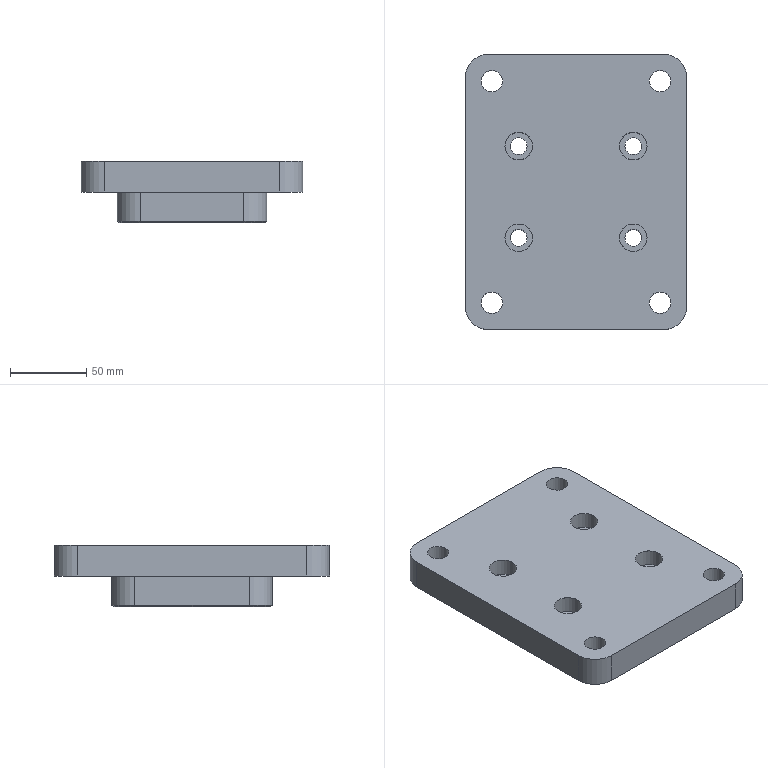NC program | NX | posted with a generic post | part box 145 x 180 x 40 mm
Whole program:
N10 G17 G21 G94 G90
(ZLEVEL_PROFILE_COPY_COPY , TOOL : D50)
N12 T02 M6
N14 G54
N16 G17 G0 G90 X-77.65 Y-31.479 S1200 M3
N18 G43 Z30. H2
N20 Z3.
N22 G94 G1 Y33.983 Z1.286 F1000.
N24 X-77.645 Y34.619 Z1.269
N26 X-77.453 Y37.973 Z1.181
N28 X-77.256 Y39.719 Z1.135
N30 X-76.807 Y42.3 Z1.067
N32 X-76.404 Y44.009 Z1.021
N34 X-75.332 Y47.446 Z0.926
N36 X-74.727 Y49.078 Z0.881
N38 X-74.17 Y50.386 Z0.844
N40 X-73.41 Y51.952 Z0.798
N42 X-72.649 Y53.443 Z0.754
N44 X-71.911 Y54.721 Z0.715
N46 X-71. Y56.126 Z0.672
N48 X-70.039 Y57.546 Z0.627
N50 X-69.127 Y58.757 Z0.587
N52 X-68.029 Y60.073 Z0.542
N54 X-66.874 Y61.393 Z0.496
N56 X-66.023 Y62.278 Z0.464
N58 X-64.752 Y63.485 Z0.418
N60 X-63.437 Y64.666 Z0.372
N62 X-62.386 Y65.526 Z0.336
N64 X-60.966 Y66.578 Z0.29
N66 X-59.562 Y67.565 Z0.245
N68 X-58.227 Y68.405 Z0.204
N70 X-56.729 Y69.243 Z0.159
N72 X-55.16 Y70.073 Z0.112
N74 X-54.177 Y70.538 Z0.084
N76 X-52.541 Y71.226 Z0.037
N78 X-50.905 Y71.862 Z-0.009
N80 X-49.631 Y72.289 Z-0.044
N82 X-47.942 Y72.768 Z-0.09
N84 X-46.24 Y73.203 Z-0.136
N86 X-44.922 Y73.473 Z-0.171
N88 X-43.187 Y73.745 Z-0.217
N90 X-41.454 Y73.955 Z-0.263
N92 X-41.399 Y73.952 Z-0.264
N94 X-38.191 Y74.15 Z-0.348
N96 X37.482 F1500.
N98 X38.098 Y74.146
N100 X41.454 Y73.955
N102 G2 X46.285 Y73.177 R50.792
N104 X50.931 Y71.837 R50.973
N106 X55.461 Y69.909 R51.3
N108 X59.617 Y67.505 R48.559
N110 X63.565 Y64.536 R48.992
N112 X67.002 Y61.233 R50.91
N114 X70.071 Y57.476 R52.422
N116 X72.739 Y53.237 R48.793
N118 X74.717 Y49.055 R51.479
N120 X76.265 Y44.454 R45.675
N122 X77.25 Y39.651 R51.44
N124 X77.65 Y34.561 R51.431
N126 G1 Y-33.983
N128 X77.645 Y-34.619
N130 X77.453 Y-37.973
N132 G2 X76.676 Y-42.79 R51.415
N134 X75.338 Y-47.427 R48.578
N136 X73.402 Y-51.973 R50.581
N138 X71. Y-56.126 R48.02
N140 X68.029 Y-60.073 R48.931
N142 X64.752 Y-63.485 R51.227
N144 X60.966 Y-66.578 R52.05
N146 X56.729 Y-69.243 R49.085
N148 X52.541 Y-71.226 R52.699
N150 X47.942 Y-72.768 R50.448
N152 X43.187 Y-73.745 R51.645
N154 X38.051 Y-74.15 R51.605
N156 G1 X-37.482
N158 X-38.098 Y-74.146
N160 X-41.508 Y-73.949
N162 G2 X-44.172 Y-73.572 R29.13
N164 G1 X-46.218 Y-73.184
N166 X-46.273 Y-73.18
N168 G2 X-50.931 Y-71.837 R50.129
N170 X-55.461 Y-69.909 R51.303
N172 X-59.617 Y-67.505 R48.559
N174 X-63.565 Y-64.536 R48.992
N176 X-67.002 Y-61.233 R50.91
N178 X-70.071 Y-57.476 R52.422
N180 X-72.739 Y-53.237 R48.666
N182 X-74.722 Y-49.052 R52.369
N184 X-76.265 Y-44.454 R50.233
N186 X-77.25 Y-39.651 R51.44
N188 X-77.65 Y-34.564 R51.114
N190 G1 Y33.983
N192 X-77.645 Y34.619
N194 X-77.453 Y37.973
N196 G2 X-76.404 Y44.009 R51.412
N198 G1 X-75.332 Y47.446
N200 G2 X-73.41 Y51.952 R50.488
N202 X-71. Y56.126 R46.691
N204 X-68.029 Y60.073 R48.958
N206 X-64.752 Y63.485 R51.227
N208 X-60.966 Y66.578 R52.05
N210 X-56.729 Y69.243 R49.085
N212 X-52.541 Y71.226 R52.488
N214 X-47.942 Y72.768 R51.35
N216 X-43.187 Y73.745 R51.432
N218 G1 X-41.454 Y73.955
N220 X-41.399 Y73.952
N222 X-38.191 Y74.15
N224 X-18.24 Z-0.696
N226 X37.482
N228 X38.098 Y74.146
N230 X41.454 Y73.955
N232 G2 X46.285 Y73.177 R50.276
N234 X50.931 Y71.837 R49.579
N236 X55.461 Y69.909 R48.594
N238 X59.618 Y67.505 R48.165
N240 X63.566 Y64.536 R49.232
N242 X67.002 Y61.233 R51.165
N244 X70.071 Y57.476 R52.131
N246 X72.739 Y53.238 R48.03
N248 X74.717 Y49.055 R48.681
N250 X76.265 Y44.454 R47.697
N252 X77.25 Y39.651 R51.088
N254 X77.65 Y34.555 R50.845
N256 G1 Y-33.983
N258 X77.645 Y-34.619
N260 X77.453 Y-37.973
N262 G2 X76.676 Y-42.79 R50.825
N264 X75.338 Y-47.427 R49.563
N266 X73.402 Y-51.973 R48.841
N268 X71. Y-56.126 R47.636
N270 X68.029 Y-60.074 R49.212
N272 X64.752 Y-63.485 R51.493
N274 X60.966 Y-66.578 R51.766
N276 X56.73 Y-69.243 R48.646
N278 X52.541 Y-71.226 R50.43
N280 X47.942 Y-72.768 R49.715
N282 X43.187 Y-73.745 R51.455
N284 X38.051 Y-74.15 R51.613
N286 G1 X-37.482
N288 X-38.098 Y-74.146
N290 X-41.508 Y-73.949
N292 G2 X-46.273 Y-73.18 R51.311
N294 X-50.931 Y-71.837 R49.633
N296 X-55.461 Y-69.909 R48.596
N298 X-59.618 Y-67.505 R48.165
N300 X-63.566 Y-64.536 R49.232
N302 X-67.002 Y-61.233 R51.165
N304 X-70.071 Y-57.476 R52.131
N306 X-72.739 Y-53.238 R47.874
N308 X-74.722 Y-49.052 R50.131
N310 X-76.265 Y-44.454 R49.505
N312 X-77.25 Y-39.651 R51.088
N314 X-77.65 Y-34.564 R51.082
N316 G1 Y33.983
N318 X-77.645 Y34.619
N320 X-77.453 Y37.973
N322 G2 X-76.4 Y44.021 R50.823
N324 G1 X-75.332 Y47.446
N326 G2 X-73.41 Y51.953 R47.836
N328 X-71. Y56.126 R46.431
N330 X-68.029 Y60.074 R49.234
N332 X-64.752 Y63.485 R51.493
N334 X-60.966 Y66.578 R51.766
N336 X-56.73 Y69.243 R48.646
N338 X-52.541 Y71.226 R50.415
N340 X-47.942 Y72.768 R49.662
N342 X-43.187 Y73.745 R51.268
N344 X-38.191 Y74.146 R50.048
N346 G1 X-37.36 Y74.15 Z-0.711
N348 X-36.529 Z-0.726
N350 X-18.24 Z-1.045
N352 X37.5
N354 G2 X77.65 Y34. R40.15
N356 G1 Y-34.
N358 G2 X37.5 Y-74.15 R40.15
N360 G1 X-37.5
N362 G2 X-68.212 Y-59.862 R40.15
N364 G1 X-68.281 Y-59.779
N366 G2 X-77.65 Y-34. R40.15
N368 G1 Y34.
N370 G2 X-38.191 Y74.144 R40.15
N372 G1 X-37.36 Y74.15 Z-1.059
N374 X-36.529 Z-1.074
N376 X-18.24 Z-1.393
N378 X37.5
N380 G2 X77.65 Y34. R40.15
N382 G1 Y-34.
N384 G2 X37.5 Y-74.15 R40.15
N386 G1 X-37.5
N388 G2 X-68.212 Y-59.862 R40.15
N390 G1 X-68.281 Y-59.779
N392 G2 X-77.65 Y-34. R40.15
N394 G1 Y34.
N396 G2 X-38.191 Y74.144 R40.15
N398 G1 X-37.36 Y74.15 Z-1.407
N400 X-36.529 Z-1.422
N402 X-18.24 Z-1.741
N404 X37.5
N406 G2 X77.65 Y34. R40.15
N408 G1 Y-34.
N410 G2 X37.5 Y-74.15 R40.15
N412 G1 X-37.5
N414 G2 X-68.212 Y-59.862 R40.15
N416 G1 X-68.281 Y-59.779
N418 G2 X-77.65 Y-34. R40.15
N420 G1 Y34.
N422 G2 X-38.191 Y74.144 R40.15
N424 G1 X-37.36 Y74.15 Z-1.756
N426 X-36.529 Z-1.77
N428 X-18.24 Z-2.089
N430 X37.5
N432 G2 X77.65 Y34. R40.15
N434 G1 Y-34.
N436 G2 X37.5 Y-74.15 R40.15
N438 G1 X-37.5
N440 G2 X-68.212 Y-59.862 R40.15
N442 G1 X-68.281 Y-59.779
N444 G2 X-77.65 Y-34. R40.15
N446 G1 Y34.
N448 G2 X-38.191 Y74.144 R40.15
N450 G1 X-37.36 Y74.15 Z-2.104
N452 X-36.529 Z-2.118
N454 X-18.24 Z-2.438
N456 X37.5
N458 G2 X77.65 Y34. R40.15
N460 G1 Y-34.
N462 G2 X37.5 Y-74.15 R40.15
N464 G1 X-37.5
N466 G2 X-68.212 Y-59.862 R40.15
N468 G1 X-68.281 Y-59.78
N470 G2 X-77.65 Y-34. R40.15
N472 G1 Y34.
N474 G2 X-38.191 Y74.144 R40.15
N476 G1 X-37.36 Y74.15 Z-2.452
N478 X-36.529 Z-2.467
N480 X-18.24 Z-2.786
N482 X37.5
N484 G2 X77.65 Y34. R40.15
N486 G1 Y-34.
N488 G2 X37.5 Y-74.15 R40.15
N490 G1 X-37.5
N492 G2 X-68.212 Y-59.862 R40.15
N494 G1 X-68.28 Y-59.78
N496 G2 X-77.65 Y-34. R40.15
N498 G1 Y34.
N500 G2 X-38.191 Y74.144 R40.15
N502 G1 X-37.36 Y74.15 Z-2.8
N504 X-36.529 Z-2.815
N506 X-18.24 Z-3.134
N508 X37.5
N510 G2 X77.65 Y34. R40.15
N512 G1 Y-34.
N514 G2 X37.5 Y-74.15 R40.15
N516 G1 X-37.5
N518 G2 X-68.212 Y-59.862 R40.15
N520 G1 X-68.28 Y-59.78
N522 G2 X-77.65 Y-34. R40.15
N524 G1 Y34.
N526 G2 X-38.191 Y74.144 R40.15
N528 G1 X-37.36 Y74.15 Z-3.149
N530 X-36.529 Z-3.163
N532 X-18.24 Z-3.482
N534 X37.5
N536 G2 X77.65 Y34. R40.15
N538 G1 Y-34.
N540 G2 X37.5 Y-74.15 R40.15
N542 G1 X-37.5
N544 G2 X-68.212 Y-59.862 R40.15
N546 G1 X-68.28 Y-59.78
N548 G2 X-77.65 Y-34. R40.15
N550 G1 Y34.
N552 G2 X-38.191 Y74.144 R40.15
N554 G1 X-37.36 Y74.15 Z-3.497
N556 X-36.529 Z-3.511
N558 X-18.24 Z-3.831
N560 X37.5
N562 G2 X77.65 Y34. R40.15
N564 G1 Y-34.
N566 G2 X37.5 Y-74.15 R40.15
N568 G1 X-37.5
N570 G2 X-68.28 Y-59.78 R40.15
N572 G1 X-68.528 Y-59.481
N574 G2 X-77.65 Y-34. R40.15
N576 G1 Y34.
N578 G2 X-38.191 Y74.144 R40.15
N580 G1 X-37.36 Y74.15 Z-3.845
N582 X-36.529 Z-3.86
N584 X-18.24 Z-4.179
N586 X37.5
N588 G2 X77.65 Y34. R40.15
N590 G1 Y-34.
N592 G2 X37.5 Y-74.15 R40.15
N594 G1 X-37.5
N596 G2 X-68.28 Y-59.78 R40.15
N598 G1 X-68.528 Y-59.481
N600 G2 X-77.65 Y-34. R40.15
N602 G1 Y34.
N604 G2 X-38.191 Y74.144 R40.15
N606 G1 X-37.36 Y74.15 Z-4.193
N608 X-36.529 Z-4.208
N610 X-18.24 Z-4.527
N612 X37.5
N614 G2 X77.65 Y34. R40.15
N616 G1 Y-34.
N618 G2 X37.5 Y-74.15 R40.15
N620 G1 X-37.5
N622 G2 X-68.28 Y-59.78 R40.15
N624 G1 X-68.528 Y-59.481
N626 G2 X-77.65 Y-34. R40.15
N628 G1 Y34.
N630 G2 X-38.191 Y74.144 R40.15
N632 G1 X-37.36 Y74.15 Z-4.542
N634 X-36.529 Z-4.556
N636 X-18.24 Z-4.875
N638 X37.5
N640 G2 X77.65 Y34. R40.15
N642 G1 Y-34.
N644 G2 X37.5 Y-74.15 R40.15
N646 G1 X-37.5
N648 G2 X-68.28 Y-59.78 R40.15
N650 G1 X-68.528 Y-59.481
N652 G2 X-77.65 Y-34. R40.15
N654 G1 Y34.
N656 G2 X-38.191 Y74.144 R40.15
N658 G1 X-37.36 Y74.15 Z-4.89
N660 X-36.529 Z-4.904
N662 X-18.24 Z-5.224
N664 X37.5
N666 G2 X77.65 Y34. R40.15
N668 G1 Y-34.
N670 G2 X37.5 Y-74.15 R40.15
N672 G1 X-37.5
N674 G2 X-68.28 Y-59.78 R40.15
N676 G1 X-68.528 Y-59.481
N678 G2 X-77.65 Y-34. R40.15
N680 G1 Y34.
N682 G2 X-38.191 Y74.144 R40.15
N684 G1 X-37.36 Y74.15 Z-5.238
N686 X-36.529 Z-5.253
N688 X-18.24 Z-5.572
N690 X37.5
N692 G2 X77.65 Y34. R40.15
N694 G1 Y-34.
N696 G2 X37.5 Y-74.15 R40.15
N698 G1 X-37.5
N700 G2 X-68.28 Y-59.78 R40.15
N702 G1 X-68.528 Y-59.481
N704 G2 X-77.65 Y-34. R40.15
N706 G1 Y34.
N708 G2 X-38.191 Y74.144 R40.15
N710 G1 X-37.36 Y74.15 Z-5.586
N712 X-36.529 Z-5.601
N714 X-18.24 Z-5.92
N716 X37.5
N718 G2 X77.65 Y34. R40.15
N720 G1 Y-34.
N722 G2 X37.5 Y-74.15 R40.15
N724 G1 X-37.5
N726 G2 X-68.28 Y-59.78 R40.15
N728 G1 X-68.528 Y-59.481
N730 G2 X-77.65 Y-34. R40.15
N732 G1 Y34.
N734 G2 X-38.191 Y74.144 R40.15
N736 G1 X-37.36 Y74.15 Z-5.935
N738 X-36.529 Z-5.949
N740 X-18.24 Z-6.268
N742 X37.5
N744 G2 X77.65 Y34. R40.15
N746 G1 Y-34.
N748 G2 X37.5 Y-74.15 R40.15
N750 G1 X-37.5
N752 G2 X-68.28 Y-59.78 R40.15
N754 G1 X-68.528 Y-59.481
N756 G2 X-77.65 Y-34. R40.15
N758 G1 Y34.
N760 G2 X-38.191 Y74.144 R40.15
N762 G1 X-37.36 Y74.15 Z-6.283
N764 X-36.529 Z-6.297
N766 X-18.24 Z-6.617
N768 X37.5
N770 G2 X77.65 Y34. R40.15
N772 G1 Y-34.
N774 G2 X37.5 Y-74.15 R40.15
N776 G1 X-37.5
N778 G2 X-68.28 Y-59.78 R40.15
N780 G1 X-68.528 Y-59.481
N782 G2 X-77.65 Y-34. R40.15
N784 G1 Y34.
N786 G2 X-38.191 Y74.144 R40.15
N788 G1 X-37.36 Y74.15 Z-6.631
N790 X-36.529 Z-6.646
N792 X-18.24 Z-6.965
N794 X37.5
N796 G2 X77.65 Y34. R40.15
N798 G1 Y-34.
N800 G2 X37.5 Y-74.15 R40.15
N802 G1 X-37.5
N804 G2 X-68.28 Y-59.78 R40.15
N806 G1 X-68.528 Y-59.481
N808 G2 X-77.65 Y-34. R40.15
N810 G1 Y34.
N812 G2 X-38.191 Y74.144 R40.15
N814 G1 X-37.36 Y74.15 Z-6.979
N816 X-36.529 Z-6.994
N818 X-18.24 Z-7.313
N820 X37.5
N822 G2 X77.65 Y34. R40.15
N824 G1 Y-34.
N826 G2 X37.5 Y-74.15 R40.15
N828 G1 X-37.5
N830 G2 X-68.28 Y-59.78 R40.15
N832 G1 X-68.528 Y-59.481
N834 G2 X-77.65 Y-34. R40.15
N836 G1 Y34.
N838 G2 X-38.191 Y74.144 R40.15
N840 G1 X-37.36 Y74.15 Z-7.328
N842 X-36.529 Z-7.342
N844 X-18.24 Z-7.661
N846 X37.5
N848 G2 X77.65 Y34. R40.15
N850 G1 Y-34.
N852 G2 X37.5 Y-74.15 R40.15
N854 G1 X-37.5
N856 G2 X-68.28 Y-59.78 R40.15
N858 G1 X-68.528 Y-59.481
N860 G2 X-77.65 Y-34. R40.15
N862 G1 Y34.
N864 G2 X-38.191 Y74.144 R40.15
N866 G1 X-37.36 Y74.15 Z-7.676
N868 X-36.529 Z-7.69
N870 X-18.24 Z-8.01
N872 X37.5
N874 G2 X77.65 Y34. R40.15
N876 G1 Y-34.
N878 G2 X37.5 Y-74.15 R40.15
N880 G1 X-37.5
N882 G2 X-68.28 Y-59.78 R40.15
N884 G1 X-68.528 Y-59.481
N886 G2 X-77.65 Y-34. R40.15
N888 G1 Y34.
N890 G2 X-38.191 Y74.144 R40.15
N892 G1 X-37.36 Y74.15 Z-8.024
N894 X-36.529 Z-8.039
N896 X-18.24 Z-8.358
N898 X37.5
N900 G2 X77.65 Y34. R40.15
N902 G1 Y-34.
N904 G2 X37.5 Y-74.15 R40.15
N906 G1 X-37.5
N908 G2 X-68.28 Y-59.78 R40.15
N910 G1 X-68.528 Y-59.481
N912 G2 X-77.65 Y-34. R40.15
N914 G1 Y34.
N916 G2 X-38.191 Y74.144 R40.15
N918 G1 X-37.36 Y74.15 Z-8.372
N920 X-36.529 Z-8.387
N922 X-18.24 Z-8.706
N924 X37.5
N926 G2 X77.65 Y34. R40.15
N928 G1 Y-34.
N930 G2 X37.5 Y-74.15 R40.15
N932 G1 X-37.5
N934 G2 X-68.28 Y-59.78 R40.15
N936 G1 X-68.528 Y-59.481
N938 G2 X-77.65 Y-34. R40.15
N940 G1 Y34.
N942 G2 X-38.191 Y74.144 R40.15
N944 G1 X-37.36 Y74.15 Z-8.721
N946 X-36.529 Z-8.735
N948 X-18.24 Z-9.054
N950 X37.5
N952 G2 X77.65 Y34. R40.15
N954 G1 Y-34.
N956 G2 X37.5 Y-74.15 R40.15
N958 G1 X-37.5
N960 G2 X-68.28 Y-59.78 R40.15
N962 G1 X-68.528 Y-59.481
N964 G2 X-77.65 Y-34. R40.15
N966 G1 Y34.
N968 G2 X-38.191 Y74.144 R40.15
N970 G1 X-37.36 Y74.15 Z-9.069
N972 X-36.529 Z-9.083
N974 X-18.24 Z-9.403
N976 X37.5
N978 G2 X77.65 Y34. R40.15
N980 G1 Y-34.
N982 G2 X37.5 Y-74.15 R40.15
N984 G1 X-37.5
N986 G2 X-68.28 Y-59.78 R40.15
N988 G1 X-68.528 Y-59.481
N990 G2 X-77.65 Y-34. R40.15
N992 G1 Y34.
N994 G2 X-38.191 Y74.144 R40.15
N996 G1 X-37.36 Y74.15 Z-9.417
N998 X-36.529 Z-9.432
N1000 X-18.24 Z-9.751
N1002 X37.5
N1004 G2 X77.65 Y34. R40.15
N1006 G1 Y-34.
N1008 G2 X37.5 Y-74.15 R40.15
N1010 G1 X-37.5
N1012 G2 X-68.28 Y-59.78 R40.15
N1014 G1 X-68.528 Y-59.481
N1016 G2 X-77.65 Y-34. R40.15
N1018 G1 Y34.
N1020 G2 X-38.191 Y74.144 R40.15
N1022 G1 X-37.36 Y74.15 Z-9.765
N1024 X-36.529 Z-9.78
N1026 X-18.24 Z-10.099
N1028 X37.5
N1030 G2 X77.65 Y34. R40.15
N1032 G1 Y-34.
N1034 G2 X37.5 Y-74.15 R40.15
N1036 G1 X-37.5
N1038 G2 X-68.28 Y-59.78 R40.15
N1040 G1 X-68.528 Y-59.481
N1042 G2 X-77.65 Y-34. R40.15
N1044 G1 Y34.
N1046 G2 X-38.191 Y74.144 R40.15
N1048 G1 X-37.36 Y74.15 Z-10.114
N1050 X-36.529 Z-10.128
N1052 X-18.24 Z-10.447
N1054 X37.5
N1056 G2 X77.65 Y34. R40.15
N1058 G1 Y-34.
N1060 G2 X37.5 Y-74.15 R40.15
N1062 G1 X-37.5
N1064 G2 X-68.28 Y-59.78 R40.15
N1066 G1 X-68.528 Y-59.481
N1068 G2 X-77.65 Y-34. R40.15
N1070 G1 Y34.
N1072 G2 X-38.191 Y74.144 R40.15
N1074 G1 X-37.36 Y74.15 Z-10.462
N1076 X-36.529 Z-10.476
N1078 X-18.24 Z-10.796
N1080 X37.5
N1082 G2 X77.65 Y34. R40.15
N1084 G1 Y-34.
N1086 G2 X37.5 Y-74.15 R40.15
N1088 G1 X-37.5
N1090 G2 X-68.28 Y-59.78 R40.15
N1092 G1 X-68.528 Y-59.481
N1094 G2 X-77.65 Y-34. R40.15
N1096 G1 Y34.
N1098 G2 X-38.191 Y74.144 R40.15
N1100 G1 X-37.36 Y74.15 Z-10.81
N1102 X-36.529 Z-10.825
N1104 X-18.24 Z-11.144
N1106 X37.5
N1108 G2 X77.65 Y34. R40.15
N1110 G1 Y-34.
N1112 G2 X37.5 Y-74.15 R40.15
N1114 G1 X-37.5
N1116 G2 X-68.28 Y-59.78 R40.15
N1118 G1 X-68.528 Y-59.481
N1120 G2 X-77.65 Y-34. R40.15
N1122 G1 Y34.
N1124 G2 X-38.191 Y74.144 R40.15
N1126 G1 X-37.36 Y74.15 Z-11.158
N1128 X-36.529 Z-11.173
N1130 X-18.24 Z-11.492
N1132 X37.5
N1134 G2 X77.65 Y34. R40.15
N1136 G1 Y-34.
N1138 G2 X37.5 Y-74.15 R40.15
N1140 G1 X-37.5
N1142 G2 X-68.28 Y-59.78 R40.15
N1144 G1 X-68.528 Y-59.481
N1146 G2 X-77.65 Y-34. R40.15
N1148 G1 Y34.
N1150 G2 X-38.191 Y74.144 R40.15
N1152 G1 X-37.36 Y74.15 Z-11.507
N1154 X-36.529 Z-11.521
N1156 X-18.24 Z-11.84
N1158 X37.5
N1160 G2 X77.65 Y34. R40.15
N1162 G1 Y-34.
N1164 G2 X37.5 Y-74.15 R40.15
N1166 G1 X-37.5
N1168 G2 X-68.28 Y-59.78 R40.15
N1170 G1 X-68.528 Y-59.481
N1172 G2 X-77.65 Y-34. R40.15
N1174 G1 Y34.
N1176 G2 X-38.191 Y74.144 R40.15
N1178 G1 X-37.36 Y74.15 Z-11.855
N1180 X-36.529 Z-11.869
N1182 X-18.24 Z-12.189
N1184 X37.5
N1186 G2 X77.65 Y34. R40.15
N1188 G1 Y-34.
N1190 G2 X37.5 Y-74.15 R40.15
N1192 G1 X-37.5
N1194 G2 X-68.28 Y-59.78 R40.15
N1196 G1 X-68.528 Y-59.481
N1198 G2 X-77.65 Y-34. R40.15
N1200 G1 Y34.
N1202 G2 X-38.191 Y74.144 R40.15
N1204 G1 X-37.36 Y74.15 Z-12.203
N1206 X-36.529 Z-12.218
N1208 X-18.24 Z-12.537
N1210 X37.5
N1212 G2 X77.65 Y34. R40.15
N1214 G1 Y-34.
N1216 G2 X37.5 Y-74.15 R40.15
N1218 G1 X-37.5
N1220 G2 X-68.28 Y-59.78 R40.15
N1222 G1 X-68.528 Y-59.481
N1224 G2 X-77.65 Y-34. R40.15
N1226 G1 Y34.
N1228 G2 X-38.191 Y74.144 R40.15
N1230 G1 X-37.36 Y74.15 Z-12.551
N1232 X-36.529 Z-12.566
N1234 X-18.24 Z-12.885
N1236 X37.5
N1238 G2 X77.65 Y34. R40.15
N1240 G1 Y-34.
N1242 G2 X37.5 Y-74.15 R40.15
N1244 G1 X-37.5
N1246 G2 X-68.28 Y-59.781 R40.15
N1248 G1 X-68.528 Y-59.481
N1250 G2 X-77.65 Y-34. R40.15
N1252 G1 Y34.
N1254 G2 X-38.191 Y74.144 R40.15
N1256 G1 X-37.36 Y74.15 Z-12.9
N1258 X-36.529 Z-12.914
N1260 X-18.24 Z-13.233
N1262 X37.5
N1264 G2 X77.65 Y34. R40.15
N1266 G1 Y-34.
N1268 G2 X37.5 Y-74.15 R40.15
N1270 G1 X-37.5
N1272 G2 X-68.28 Y-59.781 R40.15
N1274 G1 X-68.528 Y-59.481
N1276 G2 X-77.65 Y-34. R40.15
N1278 G1 Y34.
N1280 G2 X-38.191 Y74.144 R40.15
N1282 G1 X-37.36 Y74.15 Z-13.248
N1284 X-36.529 Z-13.262
N1286 X-18.24 Z-13.582
N1288 X37.5
N1290 G2 X77.65 Y34. R40.15
N1292 G1 Y-34.
N1294 G2 X37.5 Y-74.15 R40.15
N1296 G1 X-37.5
N1298 G2 X-68.28 Y-59.781 R40.15
N1300 G1 X-68.528 Y-59.481
N1302 G2 X-77.65 Y-34. R40.15
N1304 G1 Y34.
N1306 G2 X-38.191 Y74.144 R40.15
N1308 G1 X-37.36 Y74.15 Z-13.596
N1310 X-36.529 Z-13.611
N1312 X-18.24 Z-13.93
N1314 X37.5
N1316 G2 X77.65 Y34. R40.15
N1318 G1 Y-34.
N1320 G2 X37.5 Y-74.15 R40.15
N1322 G1 X-37.5
N1324 G2 X-68.28 Y-59.781 R40.15
N1326 G1 X-68.528 Y-59.481
N1328 G2 X-77.65 Y-34. R40.15
N1330 G1 Y34.
N1332 G2 X-38.191 Y74.144 R40.15
N1334 G1 X-37.36 Y74.15 Z-13.944
N1336 X-36.529 Z-13.959
N1338 X-18.24 Z-14.278
N1340 X37.5
N1342 G2 X77.65 Y34. R40.15
N1344 G1 Y-34.
N1346 G2 X37.5 Y-74.15 R40.15
N1348 G1 X-37.5
N1350 G2 X-68.28 Y-59.781 R40.15
N1352 G1 X-68.528 Y-59.481
N1354 G2 X-77.65 Y-34. R40.15
N1356 G1 Y34.
N1358 G2 X-38.191 Y74.144 R40.15
N1360 G1 X-37.36 Y74.15 Z-14.293
N1362 X-36.529 Z-14.307
N1364 X-18.24 Z-14.626
N1366 X37.5
N1368 G2 X77.65 Y34. R40.15
N1370 G1 Y-34.
N1372 G2 X37.5 Y-74.15 R40.15
N1374 G1 X-37.5
N1376 G2 X-68.28 Y-59.781 R40.15
N1378 G1 X-68.528 Y-59.481
N1380 G2 X-77.65 Y-34. R40.15
N1382 G1 Y34.
N1384 G2 X-38.191 Y74.144 R40.15
N1386 G1 X-37.36 Y74.15 Z-14.641
N1388 X-36.529 Z-14.655
N1390 X-18.24 Z-14.975
N1392 X37.5
N1394 G2 X77.65 Y34. R40.15
N1396 G1 Y-34.
N1398 G2 X37.5 Y-74.15 R40.15
N1400 G1 X-37.5
N1402 G2 X-68.279 Y-59.781 R40.15
N1404 G1 X-68.528 Y-59.481
N1406 G2 X-77.65 Y-34. R40.15
N1408 G1 Y34.
N1410 G2 X-38.191 Y74.144 R40.15
N1412 G1 X-37.36 Y74.15 Z-14.989
N1414 X-36.529 Z-15.004
N1416 X-18.24 Z-15.323
N1418 X37.5
N1420 G2 X77.65 Y34. R40.15
N1422 G1 Y-34.
N1424 G2 X37.5 Y-74.15 R40.15
N1426 G1 X-37.5
N1428 G2 X-68.279 Y-59.781 R40.15
N1430 G1 X-68.528 Y-59.481
N1432 G2 X-77.65 Y-34. R40.15
N1434 G1 Y34.
N1436 G2 X-38.191 Y74.144 R40.15
N1438 G1 X-37.36 Y74.15 Z-15.337
N1440 X-36.529 Z-15.352
N1442 X-18.24 Z-15.671
N1444 X37.5
N1446 G2 X77.65 Y34. R40.15
N1448 G1 Y-34.
N1450 G2 X37.5 Y-74.15 R40.15
N1452 G1 X-37.5
N1454 G2 X-68.279 Y-59.781 R40.15
N1456 G1 X-68.528 Y-59.481
N1458 G2 X-77.65 Y-34. R40.15
N1460 G1 Y34.
N1462 G2 X-38.191 Y74.144 R40.15
N1464 G1 X-37.36 Y74.15 Z-15.686
N1466 X-36.529 Z-15.7
N1468 X-18.24 Z-16.019
N1470 X37.5
N1472 G2 X77.65 Y34. R40.15
N1474 G1 Y-34.
N1476 G2 X37.5 Y-74.15 R40.15
N1478 G1 X-37.5
N1480 G2 X-68.279 Y-59.781 R40.15
N1482 G1 X-68.528 Y-59.481
N1484 G2 X-77.65 Y-34. R40.15
N1486 G1 Y34.
N1488 G2 X-38.191 Y74.144 R40.15
N1490 G1 X-37.36 Y74.15 Z-16.034
N1492 X-36.529 Z-16.048
N1494 X-18.24 Z-16.368
N1496 X37.5
N1498 G2 X77.65 Y34. R40.15
N1500 G1 Y-34.
N1502 G2 X37.5 Y-74.15 R40.15
N1504 G1 X-37.5
N1506 G2 X-68.279 Y-59.781 R40.15
N1508 G1 X-68.528 Y-59.481
N1510 G2 X-77.65 Y-34. R40.15
N1512 G1 Y34.
N1514 G2 X-38.191 Y74.144 R40.15
N1516 G1 X-37.36 Y74.15 Z-16.382
N1518 X-36.529 Z-16.397
N1520 X-18.24 Z-16.716
N1522 X37.5
N1524 G2 X77.65 Y34. R40.15
N1526 G1 Y-34.
N1528 G2 X37.5 Y-74.15 R40.15
N1530 G1 X-37.5
N1532 G2 X-68.279 Y-59.781 R40.15
N1534 G1 X-68.528 Y-59.481
N1536 G2 X-77.65 Y-34. R40.15
N1538 G1 Y34.
N1540 G2 X-38.191 Y74.144 R40.15
N1542 G1 X-37.36 Y74.15 Z-16.73
N1544 X-36.529 Z-16.745
N1546 X-18.24 Z-17.064
N1548 X37.5
N1550 G2 X77.65 Y34. R40.15
N1552 G1 Y-34.
N1554 G2 X37.5 Y-74.15 R40.15
N1556 G1 X-37.5
N1558 G2 X-68.279 Y-59.781 R40.15
N1560 G1 X-68.528 Y-59.481
N1562 G2 X-77.65 Y-34. R40.15
N1564 G1 Y34.
N1566 G2 X-38.191 Y74.144 R40.15
N1568 G1 X-37.36 Y74.15 Z-17.079
N1570 X-36.529 Z-17.093
N1572 X-18.24 Z-17.412
N1574 X37.5
N1576 G2 X77.65 Y34. R40.15
N1578 G1 Y-34.
N1580 G2 X37.5 Y-74.15 R40.15
N1582 G1 X-37.5
N1584 G2 X-68.279 Y-59.781 R40.15
N1586 G1 X-68.528 Y-59.481
N1588 G2 X-77.65 Y-34. R40.15
N1590 G1 Y34.
N1592 G2 X-38.191 Y74.144 R40.15
N1594 G1 X-37.36 Y74.15 Z-17.427
N1596 X-36.529 Z-17.441
N1598 X-18.24 Z-17.761
N1600 X37.5
N1602 G2 X77.65 Y34. R40.15
N1604 G1 Y-34.
N1606 G2 X37.5 Y-74.15 R40.15
N1608 G1 X-37.5
N1610 G2 X-68.279 Y-59.781 R40.15
N1612 G1 X-68.528 Y-59.481
N1614 G2 X-77.65 Y-34. R40.15
N1616 G1 Y34.
N1618 G2 X-38.191 Y74.144 R40.15
N1620 G1 X-37.36 Y74.15 Z-17.775
N1622 X-36.529 Z-17.79
N1624 X-18.24 Z-18.109
N1626 X37.5
N1628 G2 X77.65 Y34. R40.15
N1630 G1 Y-34.
N1632 G2 X37.5 Y-74.15 R40.15
N1634 G1 X-37.5
N1636 G2 X-68.279 Y-59.781 R40.15
N1638 G1 X-68.528 Y-59.481
N1640 G2 X-77.65 Y-34. R40.15
N1642 G1 Y34.
N1644 G2 X-38.191 Y74.144 R40.15
N1646 G1 X-37.36 Y74.15 Z-18.123
N1648 X-36.529 Z-18.138
N1650 X-18.24 Z-18.457
N1652 X37.5
N1654 G2 X77.65 Y34. R40.15
N1656 G1 Y-34.
N1658 G2 X37.5 Y-74.15 R40.15
N1660 G1 X-37.5
N1662 G2 X-68.279 Y-59.781 R40.15
N1664 G1 X-68.528 Y-59.481
N1666 G2 X-77.65 Y-34. R40.15
N1668 G1 Y34.
N1670 G2 X-38.191 Y74.144 R40.15
N1672 G1 X-37.36 Y74.15 Z-18.472
N1674 X-36.529 Z-18.486
N1676 X-18.24 Z-18.805
N1678 X37.5
N1680 G2 X77.65 Y34. R40.15
N1682 G1 Y-34.
N1684 G2 X37.5 Y-74.15 R40.15
N1686 G1 X-37.5
N1688 G2 X-68.279 Y-59.781 R40.15
N1690 G1 X-68.528 Y-59.481
N1692 G2 X-77.65 Y-34. R40.15
N1694 G1 Y34.
N1696 G2 X-38.191 Y74.144 R40.15
N1698 G1 X-37.36 Y74.15 Z-18.82
N1700 X-36.529 Z-18.834
N1702 X-18.24 Z-19.154
N1704 X37.5
N1706 G2 X77.65 Y34. R40.15
N1708 G1 Y-34.
N1710 G2 X37.5 Y-74.15 R40.15
N1712 G1 X-37.5
N1714 G2 X-68.279 Y-59.781 R40.15
N1716 G1 X-68.528 Y-59.481
N1718 G2 X-77.65 Y-34. R40.15
N1720 G1 Y34.
N1722 G2 X-38.191 Y74.144 R40.15
N1724 G1 X-37.36 Y74.15 Z-19.168
N1726 X-36.529 Z-19.183
N1728 X-18.24 Z-19.502
N1730 X37.5
N1732 G2 X77.65 Y34. R40.15
N1734 G1 Y-34.
N1736 G2 X37.5 Y-74.15 R40.15
N1738 G1 X-37.5
N1740 G2 X-68.279 Y-59.781 R40.15
N1742 G1 X-68.528 Y-59.481
N1744 G2 X-77.65 Y-34. R40.15
N1746 G1 Y34.
N1748 G2 X-38.191 Y74.144 R40.15
N1750 G1 X-37.36 Y74.15 Z-19.516
N1752 X-36.529 Z-19.531
N1754 X-18.24 Z-19.85
N1756 X37.5
N1758 G2 X77.65 Y34. R40.15
N1760 G1 Y-34.
N1762 G2 X37.5 Y-74.15 R40.15
N1764 G1 X-37.5
N1766 G2 X-68.279 Y-59.781 R40.15
N1768 G1 X-68.528 Y-59.481
N1770 G2 X-77.65 Y-34. R40.15
N1772 G1 Y34.
N1774 G2 X-37.5 Y74.15 R40.15
N1776 G1 X-18.24
N1778 Z-16.85
N1780 G0 Z30.
N1782 M5
(FLOOR_WALL , TOOL : D10JING)
N1784 T11 M6
N1786 G54
N1788 G17 G0 G90 X-92.625 Y72.277 S5000 M3
N1790 G43 Z30. H11
N1792 Z-17.
N1794 G95 G1 Z-20. F3.
N1796 X-88.418 Y72.331
N1798 G94 X85.477 Y74.536 F1200.
N1800 G2 X90.866 Y69.677 R20.
N1802 G1 X-92.405 Y67.352
N1804 G3 X-94.391 Y62.4 R20.
N1806 G1 X93.626 Y64.784
N1808 G2 X94.859 Y59.872 R20.
N1810 G1 X-95. Y57.464
N1812 Y52.536
N1814 X-44.754 Y53.174
N1816 G3 X-52.334 Y48.15 R20.5
N1818 G1 X-95. Y47.609
N1820 Y42.681
N1822 X-55.831 Y43.178
N1824 G3 X-57.559 Y38.228 R20.5
N1826 G1 X-95. Y37.753
N1828 Y32.826
N1830 X-58. Y33.295
N1832 Y28.367
N1834 X-95. Y27.898
N1836 Y22.97
N1838 X-58. Y23.439
N1840 Y18.512
N1842 X-95. Y18.042
N1844 Y13.115
N1846 X-58. Y13.584
N1848 Y8.656
N1850 X-95. Y8.187
N1852 Y3.259
N1854 X-58. Y3.729
N1856 Y-1.199
N1858 X-95. Y-1.668
N1860 Y-6.596
N1862 X-58. Y-6.127
N1864 Y-11.055
N1866 X-95. Y-11.524
N1868 Y-16.452
N1870 X-58. Y-15.982
N1872 Y-20.91
N1874 X-95. Y-21.379
N1876 Y-26.307
N1878 X-58. Y-25.838
N1880 Y-30.765
N1882 X-95. Y-31.235
N1884 Y-36.162
N1886 X-57.93 Y-35.692
N1888 G3 X-56.906 Y-40.607 R20.5
N1890 G1 X-95. Y-41.09
N1892 Y-46.018
N1894 X-54.468 Y-45.504
N1896 G3 X-49.836 Y-50.373 R20.5
N1898 G1 X-95. Y-50.946
N1900 Y-55.873
N1902 X13.289 Y-54.5
N1904 Z-17.
N1906 G0 Z30.
N1908 X-44.754 Y53.174
N1910 Z-17.
N1912 G95 G1 Z-20. F3.
N1914 G2 X-37.5 Y54.5 R20.5
N1916 G1 X37.5
N1918 G2 X40.65 Y54.257 R20.5
N1920 G94 G1 X95. Y54.946 F1200.
N1922 Y50.018
N1924 X50.963 Y49.46
N1926 G2 X55.057 Y44.584 R20.5
N1928 G1 X95. Y45.09
N1930 Y40.163
N1932 X57.196 Y39.683
N1934 G2 X57.986 Y34.766 R20.5
N1936 G1 X95. Y35.235
N1938 Y30.307
N1940 X58. Y29.838
N1942 Y24.91
N1944 X95. Y25.38
N1946 Y20.452
N1948 X58. Y19.983
N1950 Y15.055
N1952 X95. Y15.524
N1954 Y10.596
N1956 X58. Y10.127
N1958 Y5.2
N1960 X95. Y5.669
N1962 Y0.741
N1964 X58. Y0.272
N1966 Y-4.656
N1968 X95. Y-4.187
N1970 Y-9.114
N1972 X58. Y-9.584
N1974 Y-14.511
N1976 X95. Y-14.042
N1978 Y-18.97
N1980 X58. Y-19.439
N1982 Y-24.367
N1984 X95. Y-23.898
N1986 Y-28.825
N1988 X58. Y-29.294
N1990 Y-34.
N1992 G2 X57.999 Y-34.222 R20.5
N1994 G1 X95. Y-33.753
N1996 Y-38.681
N1998 X57.34 Y-39.158
N2000 G2 X55.333 Y-44.111 R20.5
N2002 G1 X95. Y-43.608
N2004 Y-48.536
N2006 X51.377 Y-49.089
N2008 G2 X41.3 Y-54.145 R20.5
N2010 G1 X95. Y-53.464
N2012 Y-57.5
N2014 G2 X94.98 Y-58.392 R20.
N2016 G1 X-94.726 Y-60.797
N2018 G3 X-93.239 Y-65.706 R20.
N2020 G1 X94.131 Y-63.33
N2022 G2 X91.842 Y-68.287 R20.
N2024 G1 X-90.117 Y-70.594
N2026 X-93.876 Y-70.642
N2028 Z-17.
N2030 G0 Z30.
N2032 X0. Y-57.5
N2034 Z-17.
N2036 G95 G1 Z-20. F3.
N2038 Y-54.
N2040 G94 X-37.5 F1200.
N2042 G2 X-57.5 Y-34. R20.
N2044 G1 Y34.
N2046 G2 X-37.5 Y54. R20.
N2048 G1 X37.5
N2050 G2 X57.5 Y34. R20.
N2052 G1 Y-34.
N2054 G2 X37.5 Y-54. R20.
N2056 G1 X0.
N2058 Y-57.5
N2060 Z-17.
N2062 G0 Z30.
N2064 M5
(PLANAR_MILL_COPY_COPY_COPY , TOOL : D6A45)
N2066 T07 M6
N2068 G54
N2070 G17 G0 G90 X30.766 Y41.343 S7500 M3
N2072 G43 Z30. H7
N2074 Z1.5
N2076 G94 G1 Z-1.5 F1250.
N2078 G3 X30. Y41.7 R1.
N2080 X25.8 Y37.5 R4.2
N2082 X30. Y41.7 R-4.2
N2084 X29.234 Y41.343 R1.
N2086 G1 Z1.5
N2088 G0 Z30.
N2090 X-29.234
N2092 Z1.5
N2094 G1 Z-1.5
N2096 G3 X-30. Y41.7 R1.
N2098 X-34.2 Y37.5 R4.2
N2100 X-30. Y41.7 R-4.2
N2102 X-30.766 Y41.343 R1.
N2104 G1 Z1.5
N2106 G0 Z30.
N2108 X-0.766 Y50.657
N2110 Z1.5
N2112 G1 Z-1.5
N2114 G3 X0. Y50.3 R1.
N2116 G1 X37.5
N2118 G2 X53.8 Y34. R16.3
N2120 G1 Y-34.
N2122 G2 X37.5 Y-50.3 R16.3
N2124 G1 X-37.5
N2126 G2 X-53.8 Y-34. R16.3
N2128 G1 Y34.
N2130 G2 X-37.5 Y50.3 R16.3
N2132 G1 X0.
N2134 G3 X0.766 Y50.657 R1.
N2136 G1 Z1.5
N2138 G0 Z30.
N2140 X-30.766 Y-41.343
N2142 Z1.5
N2144 G1 Z-1.5
N2146 G3 X-30. Y-41.7 R1.
N2148 X-25.8 Y-37.5 R4.2
N2150 X-30. Y-41.7 R-4.2
N2152 X-29.234 Y-41.343 R1.
N2154 G1 Z1.5
N2156 G0 Z30.
N2158 X29.234
N2160 Z1.5
N2162 G1 Z-1.5
N2164 G3 X30. Y-41.7 R1.
N2166 X34.2 Y-37.5 R4.2
N2168 X30. Y-41.7 R-4.2
N2170 X30.766 Y-41.343 R1.
N2172 G1 Z1.5
N2174 G0 Z30.
(PLANAR_MILL_COPY_COPY_COPY_COPY , TOOL : D6A45)
N2176 X-77.343 Y-54.234
N2178 Z-19.
N2180 G1 Z-22.
N2182 G3 X-77.7 Y-55. R1.
N2184 X-72.5 Y-60.2 R5.2
N2186 X-77.7 Y-55. R-5.2
N2188 X-77.343 Y-55.766 R1.
N2190 G1 Z-19.
N2192 G0 Z30.
N2194 Y55.766
N2196 Z-19.
N2198 G1 Z-22.
N2200 G3 X-77.7 Y55. R1.
N2202 X-72.5 Y49.8 R5.2
N2204 X-77.7 Y55. R-5.2
N2206 X-77.343 Y54.234 R1.
N2208 G1 Z-19.
N2210 G0 Z30.
N2212 X-0.766 Y74.657
N2214 Z-19.
N2216 G1 Z-22.
N2218 G3 X0. Y74.3 R1.
N2220 G1 X75.
N2222 G2 X91.8 Y57.5 R16.8
N2224 G1 Y-57.5
N2226 G2 X75. Y-74.3 R16.8
N2228 G1 X-75.
N2230 G2 X-91.8 Y-57.5 R16.8
N2232 G1 Y57.5
N2234 G2 X-75. Y74.3 R16.8
N2236 G1 X0.
N2238 G3 X0.766 Y74.657 R1.
N2240 G1 Z-19.
N2242 G0 Z30.
N2244 X73.266 Y59.843
N2246 Z-19.
N2248 G1 Z-22.
N2250 G3 X72.5 Y60.2 R1.
N2252 X67.3 Y55. R5.2
N2254 X72.5 Y60.2 R-5.2
N2256 X71.734 Y59.843 R1.
N2258 G1 Z-19.
N2260 G0 Z30.
N2262 X77.343 Y-55.766
N2264 Z-19.
N2266 G1 Z-22.
N2268 G3 X77.7 Y-55. R1.
N2270 X72.5 Y-49.8 R5.2
N2272 X77.7 Y-55. R-5.2
N2274 X77.343 Y-54.234 R1.
N2276 G1 Z-19.
N2278 G0 Z30.
N2280 M5
N2282 M2